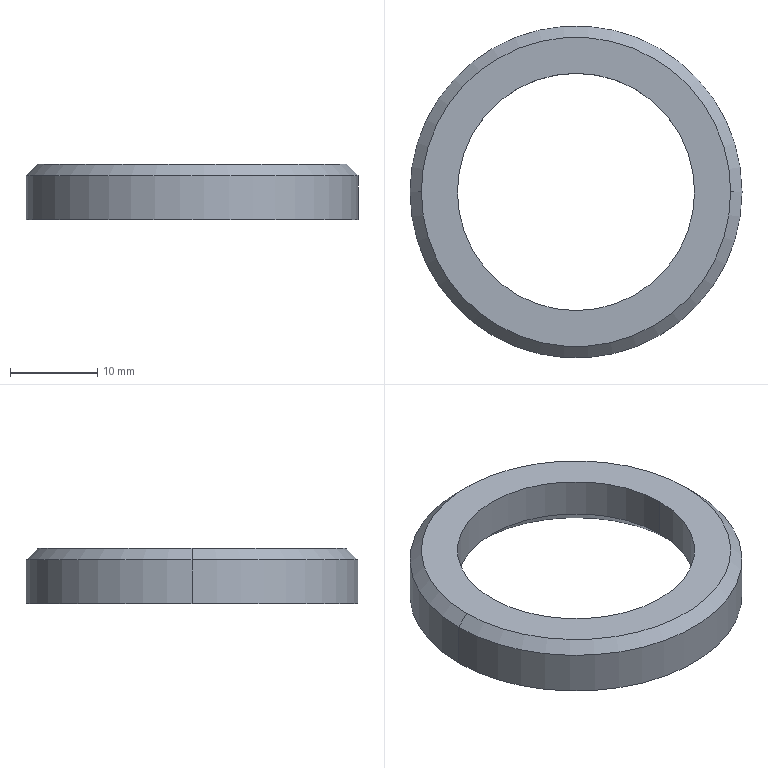Part | SolidWorks | features Chamfer 2, Extrusion 1 | 1 solid | 10 faces | box 38 x 38 x 6.3 mm | volume 3255 mm3 | cone 4 | cylinder 4 | plane 2 | commonest cylinder face diameters 27.15 x2 38 x2
STEP:
#1=CARTESIAN_POINT('',(13.575,0.,1.8));
#2=VERTEX_POINT('',#1);
#3=CARTESIAN_POINT('',(-13.575,0.,1.8));
#4=VERTEX_POINT('',#3);
#5=CARTESIAN_POINT('',(0.,0.,1.8));
#6=DIRECTION('',(0.,0.,-1.));
#7=DIRECTION('',(1.,0.,0.));
#8=AXIS2_PLACEMENT_3D('',#5,#6,#7);
#9=CIRCLE('',#8,13.575);
#10=EDGE_CURVE('',#2,#4,#9,.T.);
#11=ORIENTED_EDGE('',*,*,#10,.F.);
#12=CARTESIAN_POINT('',(15.375,0.,0.));
#13=VERTEX_POINT('',#12);
#14=CARTESIAN_POINT('',(15.375,0.,0.));
#15=DIRECTION('',(0.7071,0.,-0.7071));
#16=VECTOR('',#15,1000.);
#17=LINE('',#14,#16);
#18=EDGE_CURVE('',#2,#13,#17,.T.);
#19=ORIENTED_EDGE('',*,*,#18,.T.);
#20=CARTESIAN_POINT('',(-15.375,0.,0.));
#21=VERTEX_POINT('',#20);
#22=CARTESIAN_POINT('',(0.,0.,0.));
#23=DIRECTION('',(0.,0.,1.));
#24=DIRECTION('',(1.,0.,0.));
#25=AXIS2_PLACEMENT_3D('',#22,#23,#24);
#26=CIRCLE('',#25,15.375);
#27=EDGE_CURVE('',#21,#13,#26,.T.);
#28=ORIENTED_EDGE('',*,*,#27,.F.);
#29=CARTESIAN_POINT('',(-15.375,0.,0.));
#30=DIRECTION('',(-0.7071,0.,-0.7071));
#31=VECTOR('',#30,1000.);
#32=LINE('',#29,#31);
#33=EDGE_CURVE('',#4,#21,#32,.T.);
#34=ORIENTED_EDGE('',*,*,#33,.F.);
#35=EDGE_LOOP('',(#11,#19,#28,#34));
#36=FACE_OUTER_BOUND('',#35,.T.);
#37=CARTESIAN_POINT('',(0.,0.,0.));
#38=DIRECTION('',(0.,0.,-1.));
#39=DIRECTION('',(-1.,0.,0.));
#40=AXIS2_PLACEMENT_3D('',#37,#38,#39);
#41=CONICAL_SURFACE('',#40,15.375,0.7854);
#42=ADVANCED_FACE('',(#36),#41,.F.);
#43=CARTESIAN_POINT('',(17.7,0.,6.3));
#44=VERTEX_POINT('',#43);
#45=CARTESIAN_POINT('',(-17.7,0.,6.3));
#46=VERTEX_POINT('',#45);
#47=CARTESIAN_POINT('',(0.,0.,6.3));
#48=DIRECTION('',(0.,0.,1.));
#49=DIRECTION('',(1.,0.,0.));
#50=AXIS2_PLACEMENT_3D('',#47,#48,#49);
#51=CIRCLE('',#50,17.7);
#52=EDGE_CURVE('',#44,#46,#51,.T.);
#53=ORIENTED_EDGE('',*,*,#52,.F.);
#54=CARTESIAN_POINT('',(19.,0.,5.));
#55=VERTEX_POINT('',#54);
#56=CARTESIAN_POINT('',(17.7,0.,6.3));
#57=DIRECTION('',(0.7071,0.,-0.7071));
#58=VECTOR('',#57,1000.);
#59=LINE('',#56,#58);
#60=EDGE_CURVE('',#44,#55,#59,.T.);
#61=ORIENTED_EDGE('',*,*,#60,.T.);
#62=CARTESIAN_POINT('',(-19.,0.,5.));
#63=VERTEX_POINT('',#62);
#64=CARTESIAN_POINT('',(0.,0.,5.));
#65=DIRECTION('',(0.,0.,-1.));
#66=DIRECTION('',(1.,0.,0.));
#67=AXIS2_PLACEMENT_3D('',#64,#65,#66);
#68=CIRCLE('',#67,19.);
#69=EDGE_CURVE('',#63,#55,#68,.T.);
#70=ORIENTED_EDGE('',*,*,#69,.F.);
#71=CARTESIAN_POINT('',(-17.7,0.,6.3));
#72=DIRECTION('',(-0.7071,0.,-0.7071));
#73=VECTOR('',#72,1000.);
#74=LINE('',#71,#73);
#75=EDGE_CURVE('',#46,#63,#74,.T.);
#76=ORIENTED_EDGE('',*,*,#75,.F.);
#77=EDGE_LOOP('',(#53,#61,#70,#76));
#78=FACE_OUTER_BOUND('',#77,.T.);
#79=CARTESIAN_POINT('',(0.,0.,6.3));
#80=DIRECTION('',(0.,0.,-1.));
#81=DIRECTION('',(-1.,0.,0.));
#82=AXIS2_PLACEMENT_3D('',#79,#80,#81);
#83=CONICAL_SURFACE('',#82,17.7,0.7854);
#84=ADVANCED_FACE('',(#78),#83,.T.);
#85=CARTESIAN_POINT('',(-13.575,0.,6.3));
#86=VERTEX_POINT('',#85);
#87=CARTESIAN_POINT('',(13.575,0.,6.3));
#88=VERTEX_POINT('',#87);
#89=CARTESIAN_POINT('',(0.,0.,6.3));
#90=DIRECTION('',(0.,0.,1.));
#91=DIRECTION('',(1.,0.,0.));
#92=AXIS2_PLACEMENT_3D('',#89,#90,#91);
#93=CIRCLE('',#92,13.575);
#94=EDGE_CURVE('',#86,#88,#93,.T.);
#95=ORIENTED_EDGE('',*,*,#94,.T.);
#96=CARTESIAN_POINT('',(13.575,0.,6.3));
#97=DIRECTION('',(0.,0.,-1.));
#98=VECTOR('',#97,1000.);
#99=LINE('',#96,#98);
#100=EDGE_CURVE('',#88,#2,#99,.T.);
#101=ORIENTED_EDGE('',*,*,#100,.T.);
#102=ORIENTED_EDGE('',*,*,#10,.T.);
#103=CARTESIAN_POINT('',(-13.575,0.,6.3));
#104=DIRECTION('',(0.,0.,-1.));
#105=VECTOR('',#104,1000.);
#106=LINE('',#103,#105);
#107=EDGE_CURVE('',#86,#4,#106,.T.);
#108=ORIENTED_EDGE('',*,*,#107,.F.);
#109=EDGE_LOOP('',(#95,#101,#102,#108));
#110=FACE_OUTER_BOUND('',#109,.T.);
#111=CARTESIAN_POINT('',(0.,0.,6.3));
#112=DIRECTION('',(0.,0.,-1.));
#113=DIRECTION('',(-1.,0.,0.));
#114=AXIS2_PLACEMENT_3D('',#111,#112,#113);
#115=CYLINDRICAL_SURFACE('',#114,13.575);
#116=ADVANCED_FACE('',(#110),#115,.F.);
#117=ORIENTED_EDGE('',*,*,#69,.T.);
#118=CARTESIAN_POINT('',(19.,0.,0.));
#119=VERTEX_POINT('',#118);
#120=CARTESIAN_POINT('',(19.,0.,6.3));
#121=DIRECTION('',(0.,0.,-1.));
#122=VECTOR('',#121,1000.);
#123=LINE('',#120,#122);
#124=EDGE_CURVE('',#55,#119,#123,.T.);
#125=ORIENTED_EDGE('',*,*,#124,.T.);
#126=CARTESIAN_POINT('',(-19.,0.,0.));
#127=VERTEX_POINT('',#126);
#128=CARTESIAN_POINT('',(0.,0.,0.));
#129=DIRECTION('',(0.,0.,1.));
#130=DIRECTION('',(1.,0.,0.));
#131=AXIS2_PLACEMENT_3D('',#128,#129,#130);
#132=CIRCLE('',#131,19.);
#133=EDGE_CURVE('',#119,#127,#132,.T.);
#134=ORIENTED_EDGE('',*,*,#133,.T.);
#135=CARTESIAN_POINT('',(-19.,0.,6.3));
#136=DIRECTION('',(0.,0.,-1.));
#137=VECTOR('',#136,1000.);
#138=LINE('',#135,#137);
#139=EDGE_CURVE('',#63,#127,#138,.T.);
#140=ORIENTED_EDGE('',*,*,#139,.F.);
#141=EDGE_LOOP('',(#117,#125,#134,#140));
#142=FACE_OUTER_BOUND('',#141,.T.);
#143=CARTESIAN_POINT('',(0.,0.,6.3));
#144=DIRECTION('',(0.,0.,-1.));
#145=DIRECTION('',(-1.,0.,0.));
#146=AXIS2_PLACEMENT_3D('',#143,#144,#145);
#147=CYLINDRICAL_SURFACE('',#146,19.);
#148=ADVANCED_FACE('',(#142),#147,.T.);
#149=CARTESIAN_POINT('',(0.,0.,6.3));
#150=DIRECTION('',(0.,0.,1.));
#151=DIRECTION('',(1.,0.,0.));
#152=AXIS2_PLACEMENT_3D('',#149,#150,#151);
#153=CIRCLE('',#152,17.7);
#154=EDGE_CURVE('',#46,#44,#153,.T.);
#155=ORIENTED_EDGE('',*,*,#154,.T.);
#156=ORIENTED_EDGE('',*,*,#52,.T.);
#157=EDGE_LOOP('',(#155,#156));
#158=FACE_OUTER_BOUND('',#157,.T.);
#159=ORIENTED_EDGE('',*,*,#94,.F.);
#160=CARTESIAN_POINT('',(0.,0.,6.3));
#161=DIRECTION('',(0.,0.,1.));
#162=DIRECTION('',(1.,0.,0.));
#163=AXIS2_PLACEMENT_3D('',#160,#161,#162);
#164=CIRCLE('',#163,13.575);
#165=EDGE_CURVE('',#88,#86,#164,.T.);
#166=ORIENTED_EDGE('',*,*,#165,.F.);
#167=EDGE_LOOP('',(#159,#166));
#168=FACE_BOUND('',#167,.T.);
#169=CARTESIAN_POINT('',(0.,0.,6.3));
#170=DIRECTION('',(0.,0.,1.));
#171=DIRECTION('',(1.,0.,0.));
#172=AXIS2_PLACEMENT_3D('',#169,#170,#171);
#173=PLANE('',#172);
#174=ADVANCED_FACE('',(#158,#168),#173,.T.);
#175=ORIENTED_EDGE('',*,*,#27,.T.);
#176=CARTESIAN_POINT('',(0.,0.,0.));
#177=DIRECTION('',(0.,0.,1.));
#178=DIRECTION('',(1.,0.,0.));
#179=AXIS2_PLACEMENT_3D('',#176,#177,#178);
#180=CIRCLE('',#179,15.375);
#181=EDGE_CURVE('',#13,#21,#180,.T.);
#182=ORIENTED_EDGE('',*,*,#181,.T.);
#183=EDGE_LOOP('',(#175,#182));
#184=FACE_BOUND('',#183,.T.);
#185=CARTESIAN_POINT('',(0.,0.,0.));
#186=DIRECTION('',(0.,0.,1.));
#187=DIRECTION('',(1.,0.,0.));
#188=AXIS2_PLACEMENT_3D('',#185,#186,#187);
#189=CIRCLE('',#188,19.);
#190=EDGE_CURVE('',#127,#119,#189,.T.);
#191=ORIENTED_EDGE('',*,*,#190,.F.);
#192=ORIENTED_EDGE('',*,*,#133,.F.);
#193=EDGE_LOOP('',(#191,#192));
#194=FACE_OUTER_BOUND('',#193,.T.);
#195=CARTESIAN_POINT('',(0.,0.,0.));
#196=DIRECTION('',(0.,0.,1.));
#197=DIRECTION('',(1.,0.,0.));
#198=AXIS2_PLACEMENT_3D('',#195,#196,#197);
#199=PLANE('',#198);
#200=ADVANCED_FACE('',(#184,#194),#199,.F.);
#201=ORIENTED_EDGE('',*,*,#124,.F.);
#202=CARTESIAN_POINT('',(0.,0.,5.));
#203=DIRECTION('',(0.,0.,-1.));
#204=DIRECTION('',(1.,0.,0.));
#205=AXIS2_PLACEMENT_3D('',#202,#203,#204);
#206=CIRCLE('',#205,19.);
#207=EDGE_CURVE('',#55,#63,#206,.T.);
#208=ORIENTED_EDGE('',*,*,#207,.T.);
#209=ORIENTED_EDGE('',*,*,#139,.T.);
#210=ORIENTED_EDGE('',*,*,#190,.T.);
#211=EDGE_LOOP('',(#201,#208,#209,#210));
#212=FACE_OUTER_BOUND('',#211,.T.);
#213=CARTESIAN_POINT('',(0.,0.,6.3));
#214=DIRECTION('',(0.,0.,-1.));
#215=DIRECTION('',(-1.,0.,0.));
#216=AXIS2_PLACEMENT_3D('',#213,#214,#215);
#217=CYLINDRICAL_SURFACE('',#216,19.);
#218=ADVANCED_FACE('',(#212),#217,.T.);
#219=ORIENTED_EDGE('',*,*,#100,.F.);
#220=ORIENTED_EDGE('',*,*,#165,.T.);
#221=ORIENTED_EDGE('',*,*,#107,.T.);
#222=CARTESIAN_POINT('',(0.,0.,1.8));
#223=DIRECTION('',(0.,0.,-1.));
#224=DIRECTION('',(1.,0.,0.));
#225=AXIS2_PLACEMENT_3D('',#222,#223,#224);
#226=CIRCLE('',#225,13.575);
#227=EDGE_CURVE('',#4,#2,#226,.T.);
#228=ORIENTED_EDGE('',*,*,#227,.T.);
#229=EDGE_LOOP('',(#219,#220,#221,#228));
#230=FACE_OUTER_BOUND('',#229,.T.);
#231=CARTESIAN_POINT('',(0.,0.,6.3));
#232=DIRECTION('',(0.,0.,-1.));
#233=DIRECTION('',(-1.,0.,0.));
#234=AXIS2_PLACEMENT_3D('',#231,#232,#233);
#235=CYLINDRICAL_SURFACE('',#234,13.575);
#236=ADVANCED_FACE('',(#230),#235,.F.);
#237=ORIENTED_EDGE('',*,*,#60,.F.);
#238=ORIENTED_EDGE('',*,*,#154,.F.);
#239=ORIENTED_EDGE('',*,*,#75,.T.);
#240=ORIENTED_EDGE('',*,*,#207,.F.);
#241=EDGE_LOOP('',(#237,#238,#239,#240));
#242=FACE_OUTER_BOUND('',#241,.T.);
#243=CARTESIAN_POINT('',(0.,0.,6.3));
#244=DIRECTION('',(0.,0.,-1.));
#245=DIRECTION('',(-1.,0.,0.));
#246=AXIS2_PLACEMENT_3D('',#243,#244,#245);
#247=CONICAL_SURFACE('',#246,17.7,0.7854);
#248=ADVANCED_FACE('',(#242),#247,.T.);
#249=ORIENTED_EDGE('',*,*,#18,.F.);
#250=ORIENTED_EDGE('',*,*,#227,.F.);
#251=ORIENTED_EDGE('',*,*,#33,.T.);
#252=ORIENTED_EDGE('',*,*,#181,.F.);
#253=EDGE_LOOP('',(#249,#250,#251,#252));
#254=FACE_OUTER_BOUND('',#253,.T.);
#255=CARTESIAN_POINT('',(0.,0.,0.));
#256=DIRECTION('',(0.,0.,-1.));
#257=DIRECTION('',(-1.,0.,0.));
#258=AXIS2_PLACEMENT_3D('',#255,#256,#257);
#259=CONICAL_SURFACE('',#258,15.375,0.7854);
#260=ADVANCED_FACE('',(#254),#259,.F.);
#261=CLOSED_SHELL('',(#42,#84,#116,#148,#174,#200,#218,#236,#248,#260));
#262=MANIFOLD_SOLID_BREP('',#261);
#263=CARTESIAN_POINT('',(0.,0.,0.));
#264=DIRECTION('',(0.,0.,1.));
#265=DIRECTION('',(1.,0.,0.));
#266=AXIS2_PLACEMENT_3D('',#263,#264,#265);
#267=(LENGTH_UNIT()NAMED_UNIT(*)SI_UNIT(.MILLI.,.METRE.));
#268=UNCERTAINTY_MEASURE_WITH_UNIT(LENGTH_MEASURE(0.00001),#267,'','');
#269=(NAMED_UNIT(*)PLANE_ANGLE_UNIT()SI_UNIT($,.RADIAN.));
#270=(NAMED_UNIT(*)SI_UNIT($,.STERADIAN.)SOLID_ANGLE_UNIT());
#271=(GEOMETRIC_REPRESENTATION_CONTEXT(3)GLOBAL_UNCERTAINTY_ASSIGNED_CONTEXT((#268))GLOBAL_UNIT_ASSIGNED_CONTEXT((#267,#269,#270))REPRESENTATION_CONTEXT('',''));
#272=ADVANCED_BREP_SHAPE_REPRESENTATION('',(#262,#266),#271);